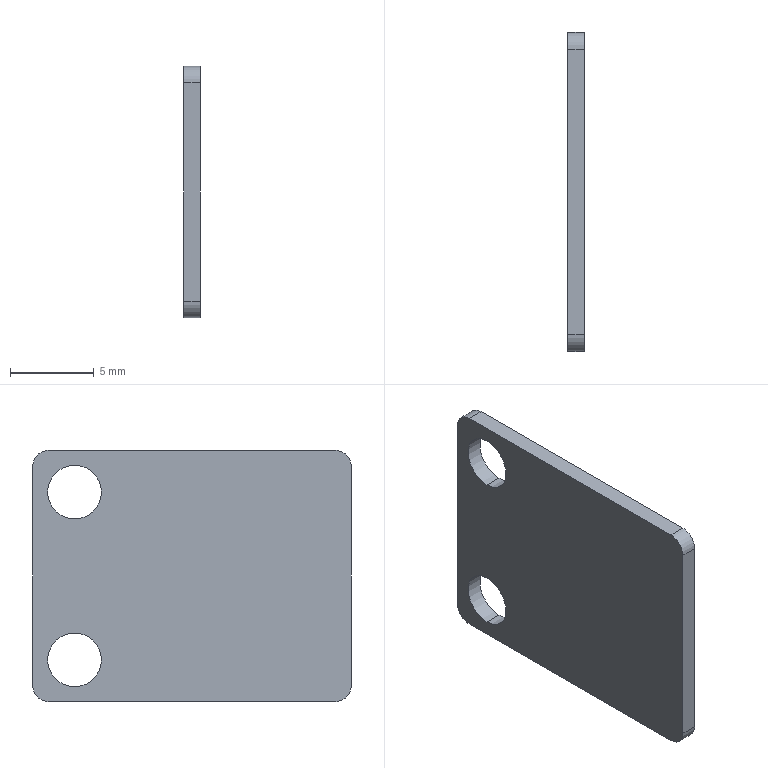Part | NX | features BREP 1 | 1 solid | 14 faces | box 1 x 19 x 15 mm | volume 268.057 mm3 | cylinder 8 | plane 6 | commonest cylinder face diameters 2 x4 3.2 x4
STEP:
#1=CARTESIAN_POINT('',(-1.,-1.,7.5));
#2=VERTEX_POINT('',#1);
#3=CARTESIAN_POINT('',(-1.,0.,6.5));
#4=VERTEX_POINT('',#3);
#5=CARTESIAN_POINT('',(-1.,-1.,6.5));
#6=DIRECTION('',(-1.,0.,0.));
#7=DIRECTION('',(0.,1.,0.));
#8=AXIS2_PLACEMENT_3D('',#5,#6,#7);
#9=CIRCLE('',#8,1.);
#10=EDGE_CURVE('',#2,#4,#9,.T.);
#11=ORIENTED_EDGE('',*,*,#10,.F.);
#12=CARTESIAN_POINT('',(0.,-1.,7.5));
#13=VERTEX_POINT('',#12);
#14=CARTESIAN_POINT('',(-1.,-1.,7.5));
#15=DIRECTION('',(-1.,0.,0.));
#16=VECTOR('',#15,1000.);
#17=LINE('',#14,#16);
#18=EDGE_CURVE('',#13,#2,#17,.T.);
#19=ORIENTED_EDGE('',*,*,#18,.F.);
#20=CARTESIAN_POINT('',(0.,0.,6.5));
#21=VERTEX_POINT('',#20);
#22=CARTESIAN_POINT('',(0.,-1.,6.5));
#23=DIRECTION('',(1.,0.,0.));
#24=DIRECTION('',(0.,1.,0.));
#25=AXIS2_PLACEMENT_3D('',#22,#23,#24);
#26=CIRCLE('',#25,1.);
#27=EDGE_CURVE('',#21,#13,#26,.T.);
#28=ORIENTED_EDGE('',*,*,#27,.F.);
#29=CARTESIAN_POINT('',(0.,0.,6.5));
#30=DIRECTION('',(1.,0.,0.));
#31=VECTOR('',#30,1000.);
#32=LINE('',#29,#31);
#33=EDGE_CURVE('',#4,#21,#32,.T.);
#34=ORIENTED_EDGE('',*,*,#33,.F.);
#35=EDGE_LOOP('',(#11,#19,#28,#34));
#36=FACE_BOUND('',#35,.T.);
#37=CARTESIAN_POINT('',(-1.,-1.,6.5));
#38=DIRECTION('',(-1.,0.,0.));
#39=DIRECTION('',(0.,-1.,0.));
#40=AXIS2_PLACEMENT_3D('',#37,#38,#39);
#41=CYLINDRICAL_SURFACE('',#40,1.);
#42=ADVANCED_FACE('',(#36),#41,.T.);
#43=CARTESIAN_POINT('',(-1.,0.,-6.5));
#44=VERTEX_POINT('',#43);
#45=CARTESIAN_POINT('',(-1.,-1.,-7.5));
#46=VERTEX_POINT('',#45);
#47=CARTESIAN_POINT('',(-1.,-1.,-6.5));
#48=DIRECTION('',(-1.,0.,0.));
#49=DIRECTION('',(0.,1.,0.));
#50=AXIS2_PLACEMENT_3D('',#47,#48,#49);
#51=CIRCLE('',#50,1.);
#52=EDGE_CURVE('',#44,#46,#51,.T.);
#53=ORIENTED_EDGE('',*,*,#52,.F.);
#54=CARTESIAN_POINT('',(0.,0.,-6.5));
#55=VERTEX_POINT('',#54);
#56=CARTESIAN_POINT('',(-1.,0.,-6.5));
#57=DIRECTION('',(-1.,0.,0.));
#58=VECTOR('',#57,1000.);
#59=LINE('',#56,#58);
#60=EDGE_CURVE('',#55,#44,#59,.T.);
#61=ORIENTED_EDGE('',*,*,#60,.F.);
#62=CARTESIAN_POINT('',(0.,-1.,-7.5));
#63=VERTEX_POINT('',#62);
#64=CARTESIAN_POINT('',(0.,-1.,-6.5));
#65=DIRECTION('',(1.,0.,0.));
#66=DIRECTION('',(0.,1.,0.));
#67=AXIS2_PLACEMENT_3D('',#64,#65,#66);
#68=CIRCLE('',#67,1.);
#69=EDGE_CURVE('',#63,#55,#68,.T.);
#70=ORIENTED_EDGE('',*,*,#69,.F.);
#71=CARTESIAN_POINT('',(0.,-1.,-7.5));
#72=DIRECTION('',(1.,0.,0.));
#73=VECTOR('',#72,1000.);
#74=LINE('',#71,#73);
#75=EDGE_CURVE('',#46,#63,#74,.T.);
#76=ORIENTED_EDGE('',*,*,#75,.F.);
#77=EDGE_LOOP('',(#53,#61,#70,#76));
#78=FACE_BOUND('',#77,.T.);
#79=CARTESIAN_POINT('',(0.,-1.,-6.5));
#80=DIRECTION('',(1.,0.,0.));
#81=DIRECTION('',(0.,1.,0.));
#82=AXIS2_PLACEMENT_3D('',#79,#80,#81);
#83=CYLINDRICAL_SURFACE('',#82,1.);
#84=ADVANCED_FACE('',(#78),#83,.T.);
#85=CARTESIAN_POINT('',(0.,-18.,7.5));
#86=VERTEX_POINT('',#85);
#87=CARTESIAN_POINT('',(0.,-19.,6.5));
#88=VERTEX_POINT('',#87);
#89=CARTESIAN_POINT('',(0.,-18.,6.5));
#90=DIRECTION('',(1.,0.,0.));
#91=DIRECTION('',(0.,1.,0.));
#92=AXIS2_PLACEMENT_3D('',#89,#90,#91);
#93=CIRCLE('',#92,1.);
#94=EDGE_CURVE('',#86,#88,#93,.T.);
#95=ORIENTED_EDGE('',*,*,#94,.F.);
#96=CARTESIAN_POINT('',(-1.,-18.,7.5));
#97=VERTEX_POINT('',#96);
#98=CARTESIAN_POINT('',(0.,-18.,7.5));
#99=DIRECTION('',(1.,0.,0.));
#100=VECTOR('',#99,1000.);
#101=LINE('',#98,#100);
#102=EDGE_CURVE('',#97,#86,#101,.T.);
#103=ORIENTED_EDGE('',*,*,#102,.F.);
#104=CARTESIAN_POINT('',(-1.,-19.,6.5));
#105=VERTEX_POINT('',#104);
#106=CARTESIAN_POINT('',(-1.,-18.,6.5));
#107=DIRECTION('',(-1.,0.,0.));
#108=DIRECTION('',(0.,1.,0.));
#109=AXIS2_PLACEMENT_3D('',#106,#107,#108);
#110=CIRCLE('',#109,1.);
#111=EDGE_CURVE('',#105,#97,#110,.T.);
#112=ORIENTED_EDGE('',*,*,#111,.F.);
#113=CARTESIAN_POINT('',(-1.,-19.,6.5));
#114=DIRECTION('',(-1.,0.,0.));
#115=VECTOR('',#114,1000.);
#116=LINE('',#113,#115);
#117=EDGE_CURVE('',#88,#105,#116,.T.);
#118=ORIENTED_EDGE('',*,*,#117,.F.);
#119=EDGE_LOOP('',(#95,#103,#112,#118));
#120=FACE_BOUND('',#119,.T.);
#121=CARTESIAN_POINT('',(0.,-18.,6.5));
#122=DIRECTION('',(1.,0.,0.));
#123=DIRECTION('',(0.,0.,-1.));
#124=AXIS2_PLACEMENT_3D('',#121,#122,#123);
#125=CYLINDRICAL_SURFACE('',#124,1.);
#126=ADVANCED_FACE('',(#120),#125,.T.);
#127=CARTESIAN_POINT('',(0.,-19.,-6.5));
#128=VERTEX_POINT('',#127);
#129=CARTESIAN_POINT('',(0.,-18.,-7.5));
#130=VERTEX_POINT('',#129);
#131=CARTESIAN_POINT('',(0.,-18.,-6.5));
#132=DIRECTION('',(1.,0.,0.));
#133=DIRECTION('',(0.,1.,0.));
#134=AXIS2_PLACEMENT_3D('',#131,#132,#133);
#135=CIRCLE('',#134,1.);
#136=EDGE_CURVE('',#128,#130,#135,.T.);
#137=ORIENTED_EDGE('',*,*,#136,.F.);
#138=CARTESIAN_POINT('',(-1.,-19.,-6.5));
#139=VERTEX_POINT('',#138);
#140=CARTESIAN_POINT('',(0.,-19.,-6.5));
#141=DIRECTION('',(1.,0.,0.));
#142=VECTOR('',#141,1000.);
#143=LINE('',#140,#142);
#144=EDGE_CURVE('',#139,#128,#143,.T.);
#145=ORIENTED_EDGE('',*,*,#144,.F.);
#146=CARTESIAN_POINT('',(-1.,-18.,-7.5));
#147=VERTEX_POINT('',#146);
#148=CARTESIAN_POINT('',(-1.,-18.,-6.5));
#149=DIRECTION('',(-1.,0.,0.));
#150=DIRECTION('',(0.,1.,0.));
#151=AXIS2_PLACEMENT_3D('',#148,#149,#150);
#152=CIRCLE('',#151,1.);
#153=EDGE_CURVE('',#147,#139,#152,.T.);
#154=ORIENTED_EDGE('',*,*,#153,.F.);
#155=CARTESIAN_POINT('',(0.,-18.,-7.5));
#156=DIRECTION('',(-1.,0.,0.));
#157=VECTOR('',#156,1000.);
#158=LINE('',#155,#157);
#159=EDGE_CURVE('',#130,#147,#158,.T.);
#160=ORIENTED_EDGE('',*,*,#159,.F.);
#161=EDGE_LOOP('',(#137,#145,#154,#160));
#162=FACE_BOUND('',#161,.T.);
#163=CARTESIAN_POINT('',(0.,-18.,-6.5));
#164=DIRECTION('',(-1.,0.,0.));
#165=DIRECTION('',(0.,0.,1.));
#166=AXIS2_PLACEMENT_3D('',#163,#164,#165);
#167=CYLINDRICAL_SURFACE('',#166,1.);
#168=ADVANCED_FACE('',(#162),#167,.T.);
#169=CARTESIAN_POINT('',(-1.,-2.5,6.6));
#170=VERTEX_POINT('',#169);
#171=CARTESIAN_POINT('',(0.,-2.5,6.6));
#172=VERTEX_POINT('',#171);
#173=CARTESIAN_POINT('',(0.,-2.5,6.6));
#174=DIRECTION('',(1.,0.,0.));
#175=VECTOR('',#174,1000.);
#176=LINE('',#173,#175);
#177=EDGE_CURVE('',#170,#172,#176,.T.);
#178=ORIENTED_EDGE('',*,*,#177,.F.);
#179=CARTESIAN_POINT('',(-1.,-2.5,3.4));
#180=VERTEX_POINT('',#179);
#181=CARTESIAN_POINT('',(-1.,-2.5,5.));
#182=DIRECTION('',(1.,0.,0.));
#183=DIRECTION('',(0.,1.,0.));
#184=AXIS2_PLACEMENT_3D('',#181,#182,#183);
#185=CIRCLE('',#184,1.6);
#186=EDGE_CURVE('',#180,#170,#185,.T.);
#187=ORIENTED_EDGE('',*,*,#186,.F.);
#188=CARTESIAN_POINT('',(0.,-2.5,3.4));
#189=VERTEX_POINT('',#188);
#190=CARTESIAN_POINT('',(0.,-2.5,3.4));
#191=DIRECTION('',(1.,0.,0.));
#192=VECTOR('',#191,1000.);
#193=LINE('',#190,#192);
#194=EDGE_CURVE('',#180,#189,#193,.T.);
#195=ORIENTED_EDGE('',*,*,#194,.T.);
#196=CARTESIAN_POINT('',(0.,-2.5,5.));
#197=DIRECTION('',(1.,0.,0.));
#198=DIRECTION('',(0.,0.,-1.));
#199=AXIS2_PLACEMENT_3D('',#196,#197,#198);
#200=CIRCLE('',#199,1.6);
#201=EDGE_CURVE('',#189,#172,#200,.T.);
#202=ORIENTED_EDGE('',*,*,#201,.T.);
#203=EDGE_LOOP('',(#178,#187,#195,#202));
#204=FACE_BOUND('',#203,.T.);
#205=CARTESIAN_POINT('',(0.,-2.5,5.));
#206=DIRECTION('',(1.,0.,0.));
#207=DIRECTION('',(0.,0.,-1.));
#208=AXIS2_PLACEMENT_3D('',#205,#206,#207);
#209=CYLINDRICAL_SURFACE('',#208,1.6);
#210=ADVANCED_FACE('',(#204),#209,.F.);
#211=CARTESIAN_POINT('',(-1.,-2.5,-3.4));
#212=VERTEX_POINT('',#211);
#213=CARTESIAN_POINT('',(0.,-2.5,-3.4));
#214=VERTEX_POINT('',#213);
#215=CARTESIAN_POINT('',(0.,-2.5,-3.4));
#216=DIRECTION('',(1.,0.,0.));
#217=VECTOR('',#216,1000.);
#218=LINE('',#215,#217);
#219=EDGE_CURVE('',#212,#214,#218,.T.);
#220=ORIENTED_EDGE('',*,*,#219,.F.);
#221=CARTESIAN_POINT('',(-1.,-2.5,-6.6));
#222=VERTEX_POINT('',#221);
#223=CARTESIAN_POINT('',(-1.,-2.5,-5.));
#224=DIRECTION('',(1.,0.,0.));
#225=DIRECTION('',(0.,1.,0.));
#226=AXIS2_PLACEMENT_3D('',#223,#224,#225);
#227=CIRCLE('',#226,1.6);
#228=EDGE_CURVE('',#222,#212,#227,.T.);
#229=ORIENTED_EDGE('',*,*,#228,.F.);
#230=CARTESIAN_POINT('',(0.,-2.5,-6.6));
#231=VERTEX_POINT('',#230);
#232=CARTESIAN_POINT('',(0.,-2.5,-6.6));
#233=DIRECTION('',(1.,0.,0.));
#234=VECTOR('',#233,1000.);
#235=LINE('',#232,#234);
#236=EDGE_CURVE('',#222,#231,#235,.T.);
#237=ORIENTED_EDGE('',*,*,#236,.T.);
#238=CARTESIAN_POINT('',(0.,-2.5,-5.));
#239=DIRECTION('',(1.,0.,0.));
#240=DIRECTION('',(0.,0.,-1.));
#241=AXIS2_PLACEMENT_3D('',#238,#239,#240);
#242=CIRCLE('',#241,1.6);
#243=EDGE_CURVE('',#231,#214,#242,.T.);
#244=ORIENTED_EDGE('',*,*,#243,.T.);
#245=EDGE_LOOP('',(#220,#229,#237,#244));
#246=FACE_BOUND('',#245,.T.);
#247=CARTESIAN_POINT('',(0.,-2.5,-5.));
#248=DIRECTION('',(1.,0.,0.));
#249=DIRECTION('',(0.,0.,-1.));
#250=AXIS2_PLACEMENT_3D('',#247,#248,#249);
#251=CYLINDRICAL_SURFACE('',#250,1.6);
#252=ADVANCED_FACE('',(#246),#251,.F.);
#253=CARTESIAN_POINT('',(0.,0.,-7.5));
#254=DIRECTION('',(0.,-1.,0.));
#255=VECTOR('',#254,1000.);
#256=LINE('',#253,#255);
#257=EDGE_CURVE('',#63,#130,#256,.T.);
#258=ORIENTED_EDGE('',*,*,#257,.T.);
#259=ORIENTED_EDGE('',*,*,#159,.T.);
#260=CARTESIAN_POINT('',(-1.,0.,-7.5));
#261=DIRECTION('',(0.,-1.,0.));
#262=VECTOR('',#261,1000.);
#263=LINE('',#260,#262);
#264=EDGE_CURVE('',#46,#147,#263,.T.);
#265=ORIENTED_EDGE('',*,*,#264,.F.);
#266=ORIENTED_EDGE('',*,*,#75,.T.);
#267=EDGE_LOOP('',(#258,#259,#265,#266));
#268=FACE_BOUND('',#267,.T.);
#269=CARTESIAN_POINT('',(0.,0.,-7.5));
#270=DIRECTION('',(0.,0.,-1.));
#271=DIRECTION('',(-1.,0.,0.));
#272=AXIS2_PLACEMENT_3D('',#269,#270,#271);
#273=PLANE('',#272);
#274=ADVANCED_FACE('',(#268),#273,.T.);
#275=CARTESIAN_POINT('',(-1.,0.,7.5));
#276=DIRECTION('',(0.,-1.,0.));
#277=VECTOR('',#276,1000.);
#278=LINE('',#275,#277);
#279=EDGE_CURVE('',#2,#97,#278,.T.);
#280=ORIENTED_EDGE('',*,*,#279,.T.);
#281=ORIENTED_EDGE('',*,*,#102,.T.);
#282=CARTESIAN_POINT('',(0.,0.,7.5));
#283=DIRECTION('',(0.,-1.,0.));
#284=VECTOR('',#283,1000.);
#285=LINE('',#282,#284);
#286=EDGE_CURVE('',#13,#86,#285,.T.);
#287=ORIENTED_EDGE('',*,*,#286,.F.);
#288=ORIENTED_EDGE('',*,*,#18,.T.);
#289=EDGE_LOOP('',(#280,#281,#287,#288));
#290=FACE_BOUND('',#289,.T.);
#291=CARTESIAN_POINT('',(0.,0.,7.5));
#292=DIRECTION('',(0.,0.,-1.));
#293=DIRECTION('',(-1.,0.,0.));
#294=AXIS2_PLACEMENT_3D('',#291,#292,#293);
#295=PLANE('',#294);
#296=ADVANCED_FACE('',(#290),#295,.F.);
#297=CARTESIAN_POINT('',(0.,0.,7.5));
#298=DIRECTION('',(0.,0.,-1.));
#299=VECTOR('',#298,1000.);
#300=LINE('',#297,#299);
#301=EDGE_CURVE('',#21,#55,#300,.T.);
#302=ORIENTED_EDGE('',*,*,#301,.T.);
#303=ORIENTED_EDGE('',*,*,#60,.T.);
#304=CARTESIAN_POINT('',(-1.,0.,7.5));
#305=DIRECTION('',(0.,0.,-1.));
#306=VECTOR('',#305,1000.);
#307=LINE('',#304,#306);
#308=EDGE_CURVE('',#4,#44,#307,.T.);
#309=ORIENTED_EDGE('',*,*,#308,.F.);
#310=ORIENTED_EDGE('',*,*,#33,.T.);
#311=EDGE_LOOP('',(#302,#303,#309,#310));
#312=FACE_BOUND('',#311,.T.);
#313=CARTESIAN_POINT('',(-1.,0.,7.5));
#314=DIRECTION('',(0.,1.,0.));
#315=DIRECTION('',(-1.,0.,0.));
#316=AXIS2_PLACEMENT_3D('',#313,#314,#315);
#317=PLANE('',#316);
#318=ADVANCED_FACE('',(#312),#317,.T.);
#319=CARTESIAN_POINT('',(0.,-19.,7.5));
#320=DIRECTION('',(0.,0.,-1.));
#321=VECTOR('',#320,1000.);
#322=LINE('',#319,#321);
#323=EDGE_CURVE('',#88,#128,#322,.T.);
#324=ORIENTED_EDGE('',*,*,#323,.T.);
#325=ORIENTED_EDGE('',*,*,#136,.T.);
#326=ORIENTED_EDGE('',*,*,#257,.F.);
#327=ORIENTED_EDGE('',*,*,#69,.T.);
#328=ORIENTED_EDGE('',*,*,#301,.F.);
#329=ORIENTED_EDGE('',*,*,#27,.T.);
#330=ORIENTED_EDGE('',*,*,#286,.T.);
#331=ORIENTED_EDGE('',*,*,#94,.T.);
#332=EDGE_LOOP('',(#324,#325,#326,#327,#328,#329,#330,#331));
#333=FACE_BOUND('',#332,.T.);
#334=ORIENTED_EDGE('',*,*,#243,.F.);
#335=CARTESIAN_POINT('',(0.,-2.5,-5.));
#336=DIRECTION('',(1.,0.,0.));
#337=DIRECTION('',(0.,0.,-1.));
#338=AXIS2_PLACEMENT_3D('',#335,#336,#337);
#339=CIRCLE('',#338,1.6);
#340=EDGE_CURVE('',#214,#231,#339,.T.);
#341=ORIENTED_EDGE('',*,*,#340,.F.);
#342=EDGE_LOOP('',(#334,#341));
#343=FACE_BOUND('',#342,.T.);
#344=ORIENTED_EDGE('',*,*,#201,.F.);
#345=CARTESIAN_POINT('',(0.,-2.5,5.));
#346=DIRECTION('',(1.,0.,0.));
#347=DIRECTION('',(0.,0.,-1.));
#348=AXIS2_PLACEMENT_3D('',#345,#346,#347);
#349=CIRCLE('',#348,1.6);
#350=EDGE_CURVE('',#172,#189,#349,.T.);
#351=ORIENTED_EDGE('',*,*,#350,.F.);
#352=EDGE_LOOP('',(#344,#351));
#353=FACE_BOUND('',#352,.T.);
#354=CARTESIAN_POINT('',(0.,0.,7.5));
#355=DIRECTION('',(1.,0.,0.));
#356=DIRECTION('',(0.,1.,0.));
#357=AXIS2_PLACEMENT_3D('',#354,#355,#356);
#358=PLANE('',#357);
#359=ADVANCED_FACE('',(#333,#343,#353),#358,.T.);
#360=CARTESIAN_POINT('',(-1.,-19.,7.5));
#361=DIRECTION('',(0.,0.,-1.));
#362=VECTOR('',#361,1000.);
#363=LINE('',#360,#362);
#364=EDGE_CURVE('',#105,#139,#363,.T.);
#365=ORIENTED_EDGE('',*,*,#364,.T.);
#366=ORIENTED_EDGE('',*,*,#144,.T.);
#367=ORIENTED_EDGE('',*,*,#323,.F.);
#368=ORIENTED_EDGE('',*,*,#117,.T.);
#369=EDGE_LOOP('',(#365,#366,#367,#368));
#370=FACE_BOUND('',#369,.T.);
#371=CARTESIAN_POINT('',(0.,-19.,7.5));
#372=DIRECTION('',(0.,-1.,0.));
#373=DIRECTION('',(0.,0.,-1.));
#374=AXIS2_PLACEMENT_3D('',#371,#372,#373);
#375=PLANE('',#374);
#376=ADVANCED_FACE('',(#370),#375,.T.);
#377=ORIENTED_EDGE('',*,*,#264,.T.);
#378=ORIENTED_EDGE('',*,*,#153,.T.);
#379=ORIENTED_EDGE('',*,*,#364,.F.);
#380=ORIENTED_EDGE('',*,*,#111,.T.);
#381=ORIENTED_EDGE('',*,*,#279,.F.);
#382=ORIENTED_EDGE('',*,*,#10,.T.);
#383=ORIENTED_EDGE('',*,*,#308,.T.);
#384=ORIENTED_EDGE('',*,*,#52,.T.);
#385=EDGE_LOOP('',(#377,#378,#379,#380,#381,#382,#383,#384));
#386=FACE_BOUND('',#385,.T.);
#387=ORIENTED_EDGE('',*,*,#228,.T.);
#388=CARTESIAN_POINT('',(-1.,-2.5,-5.));
#389=DIRECTION('',(1.,0.,0.));
#390=DIRECTION('',(0.,1.,0.));
#391=AXIS2_PLACEMENT_3D('',#388,#389,#390);
#392=CIRCLE('',#391,1.6);
#393=EDGE_CURVE('',#212,#222,#392,.T.);
#394=ORIENTED_EDGE('',*,*,#393,.T.);
#395=EDGE_LOOP('',(#387,#394));
#396=FACE_BOUND('',#395,.T.);
#397=ORIENTED_EDGE('',*,*,#186,.T.);
#398=CARTESIAN_POINT('',(-1.,-2.5,5.));
#399=DIRECTION('',(1.,0.,0.));
#400=DIRECTION('',(0.,1.,0.));
#401=AXIS2_PLACEMENT_3D('',#398,#399,#400);
#402=CIRCLE('',#401,1.6);
#403=EDGE_CURVE('',#170,#180,#402,.T.);
#404=ORIENTED_EDGE('',*,*,#403,.T.);
#405=EDGE_LOOP('',(#397,#404));
#406=FACE_BOUND('',#405,.T.);
#407=CARTESIAN_POINT('',(-1.,0.,7.5));
#408=DIRECTION('',(1.,0.,0.));
#409=DIRECTION('',(0.,1.,0.));
#410=AXIS2_PLACEMENT_3D('',#407,#408,#409);
#411=PLANE('',#410);
#412=ADVANCED_FACE('',(#386,#396,#406),#411,.F.);
#413=ORIENTED_EDGE('',*,*,#393,.F.);
#414=ORIENTED_EDGE('',*,*,#219,.T.);
#415=ORIENTED_EDGE('',*,*,#340,.T.);
#416=ORIENTED_EDGE('',*,*,#236,.F.);
#417=EDGE_LOOP('',(#413,#414,#415,#416));
#418=FACE_BOUND('',#417,.T.);
#419=CARTESIAN_POINT('',(0.,-2.5,-5.));
#420=DIRECTION('',(1.,0.,0.));
#421=DIRECTION('',(0.,0.,-1.));
#422=AXIS2_PLACEMENT_3D('',#419,#420,#421);
#423=CYLINDRICAL_SURFACE('',#422,1.6);
#424=ADVANCED_FACE('',(#418),#423,.F.);
#425=ORIENTED_EDGE('',*,*,#403,.F.);
#426=ORIENTED_EDGE('',*,*,#177,.T.);
#427=ORIENTED_EDGE('',*,*,#350,.T.);
#428=ORIENTED_EDGE('',*,*,#194,.F.);
#429=EDGE_LOOP('',(#425,#426,#427,#428));
#430=FACE_BOUND('',#429,.T.);
#431=CARTESIAN_POINT('',(0.,-2.5,5.));
#432=DIRECTION('',(1.,0.,0.));
#433=DIRECTION('',(0.,0.,-1.));
#434=AXIS2_PLACEMENT_3D('',#431,#432,#433);
#435=CYLINDRICAL_SURFACE('',#434,1.6);
#436=ADVANCED_FACE('',(#430),#435,.F.);
#437=CLOSED_SHELL('',(#42,#84,#126,#168,#210,#252,#274,#296,#318,#359,#376,#412,#424,#436));
#438=MANIFOLD_SOLID_BREP('',#437);
#439=(LENGTH_UNIT()NAMED_UNIT(*)SI_UNIT(.MILLI.,.METRE.));
#440=UNCERTAINTY_MEASURE_WITH_UNIT(LENGTH_MEASURE(0.00001),#439,'','');
#441=(NAMED_UNIT(*)PLANE_ANGLE_UNIT()SI_UNIT($,.RADIAN.));
#442=(NAMED_UNIT(*)SI_UNIT($,.STERADIAN.)SOLID_ANGLE_UNIT());
#443=(GEOMETRIC_REPRESENTATION_CONTEXT(3)GLOBAL_UNCERTAINTY_ASSIGNED_CONTEXT((#440))GLOBAL_UNIT_ASSIGNED_CONTEXT((#439,#441,#442))REPRESENTATION_CONTEXT('',''));
#444=ADVANCED_BREP_SHAPE_REPRESENTATION('',(#438),#443);